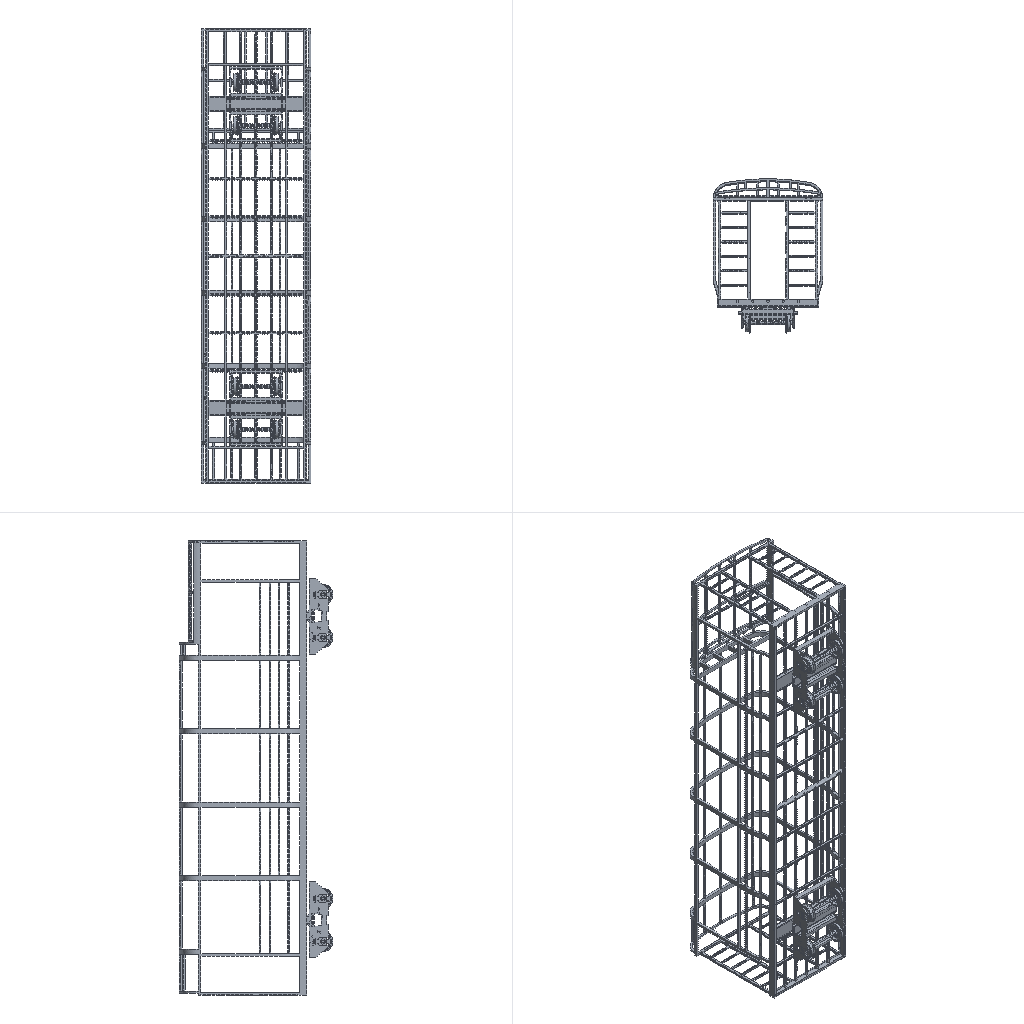Simulation study | ansys workbench
Set-up summary:
category,name,step,type,value,unit,region
solver,ansys_workbench
units,mm-N-s-tonne (MPa),,stated,"/units,MPA"
analysis,LS1,,static
load_step,LS1,LS1,static,nsubst=1; time=1
mesh,nodes,,,844923
mesh,elements,,,483421
element_type,SOLID187,,,440747
element_type,CONTA174,,,27682
element_type,TARGE170,,,10972
element_type,SOLID186,,,4020
material,Structural Steel,,E,200000,tonne s^-2 mm^-1
material,Structural Steel,,nu,0.3
material,Structural Steel,,density,7.85e-09,tonne mm^-3
material,Structural Steel,,conductivity,60.5,tonne mm s^-3 C^-1
material,Structural Steel,,specific_heat,4.34e+08,mm^2 s^-2 C^-1
material,Structural Steel,,cte,1.2e-05,C^-1
material,Structural Steel,,permeability,10000
material,Structural Steel,,resistivity,0.00017,ohm mm
load,,LS1,force,"13770 [dir=(-1, 0, 0) n=3]",,all
load,ACEL,LS1,gravity (ACEL; gravity acts opposite),"9806.65 [dir=(0, -1, 0)]",,all
bc,Constant Zero Displacement X,model,fixed,[dofs=UX],,_DISPZEROUX
bc,Constant Zero Displacement Y,model,fixed,[dofs=UY],,_DISPZEROUY
bc,Constant Zero Displacement Z,model,fixed,[dofs=UZ],,_DISPZEROUZ
contact,Contact Region 10,,bonded (always),element=CONTA174
contact,Contact Region 11,,bonded (always),element=CONTA174
contact,Contact Region 12,,bonded (always),element=CONTA174
contact,Contact Region 13,,bonded (always),element=CONTA174
contact,Contact Region 14,,bonded (always),element=CONTA174
contact,Contact Region 15,,bonded (always),element=CONTA174
contact,Contact Region 16,,bonded (always),element=CONTA174
contact,Contact Region 17,,bonded (always),element=CONTA174
contact,Contact Region 18,,bonded (always),element=CONTA174
contact,Contact Region 19,,bonded (always),element=CONTA174
contact,Contact Region 20,,bonded (always),element=CONTA174
contact,Contact Region 21,,bonded (always),element=CONTA174
contact,Contact Region 22,,bonded (always),element=CONTA174
contact,Contact Region 23,,bonded (always),element=CONTA174
contact,Contact Region 24,,bonded (always),element=CONTA174
contact,Contact Region 25,,bonded (always),element=CONTA174
contact,Contact Region 26,,bonded (always),element=CONTA174
contact,Contact Region 27,,bonded (always),element=CONTA174
contact,Contact Region 28,,bonded (always),element=CONTA174
contact,Contact Region 29,,bonded (always),element=CONTA174
contact,Contact Region 30,,bonded (always),element=CONTA174
contact,Contact Region 31,,bonded (always),element=CONTA174
contact,Contact Region 32,,bonded (always),element=CONTA174
contact,Contact Region 33,,bonded (always),element=CONTA174
contact,Contact Region 34,,bonded (always),element=CONTA174
contact,Contact Region 35,,bonded (always),element=CONTA174
contact,Contact Region 36,,bonded (always),element=CONTA174
contact,Contact Region 37,,bonded (always),element=CONTA174
contact,Contact Region 38,,bonded (always),element=CONTA174
contact,Contact Region 39,,bonded (always),element=CONTA174
contact,Contact Region 40,,bonded (always),element=CONTA174
contact,Contact Region 41,,bonded (always),element=CONTA174
contact,Contact Region 42,,bonded (always),element=CONTA174
contact,Contact Region 43,,bonded (always),element=CONTA174
contact,Contact Region 44,,bonded (always),element=CONTA174
contact,Contact Region 45,,bonded (always),element=CONTA174
contact,Contact Region 46,,bonded (always),element=CONTA174
contact,Contact Region 47,,bonded (always),element=CONTA174
contact,Contact Region 48,,bonded (always),element=CONTA174
contact,Contact Region 49,,bonded (always),element=CONTA174
contact,Contact Region 50,,bonded (always),element=CONTA174
contact,Contact Region 51,,bonded (always),element=CONTA174
contact,Contact Region 52,,bonded (always),element=CONTA174
contact,Contact Region 53,,bonded (always),element=CONTA174
contact,Contact Region 54,,bonded (always),element=CONTA174
contact,Contact Region 55,,bonded (always),element=CONTA174
contact,Contact Region 56,,bonded (always),element=CONTA174
contact,Contact Region 57,,bonded (always),element=CONTA174
contact,Contact Region 58,,bonded (always),element=CONTA174
contact,Contact Region 59,,bonded (always),element=CONTA174
contact,Contact Region 60,,bonded (always),element=CONTA174
contact,Contact Region 61,,bonded (always),element=CONTA174
contact,Contact Region 62,,bonded (always),element=CONTA174
contact,Contact Region 63,,bonded (always),element=CONTA174
contact,Contact Region 64,,bonded (always),element=CONTA174
contact,Contact Region 65,,bonded (always),element=CONTA174
contact,Contact Region 66,,bonded (always),element=CONTA174
contact,Contact Region 67,,bonded (always),element=CONTA174
contact,Contact Region 68,,bonded (always),element=CONTA174
contact,Contact Region 69,,bonded (always),element=CONTA174
contact,Contact Region 70,,bonded (always),element=CONTA174
contact,Contact Region 71,,bonded (always),element=CONTA174
contact,Contact Region 72,,bonded (always),element=CONTA174
contact,Contact Region 73,,bonded (always),element=CONTA174
contact,Contact Region 74,,bonded (always),element=CONTA174
contact,Contact Region 75,,bonded (always),element=CONTA174
contact,Contact Region 76,,bonded (always),element=CONTA174
contact,Contact Region 77,,bonded (always),element=CONTA174
contact,Contact Region 78,,bonded (always),element=CONTA174
contact,Contact Region 79,,bonded (always),element=CONTA174
contact,Contact Region 80,,bonded (always),element=CONTA174
contact,Contact Region 81,,bonded (always),element=CONTA174
contact,Contact Region 82,,bonded (always),element=CONTA174
contact,Contact Region 83,,bonded (always),element=CONTA174
contact,Contact Region 84,,bonded (always),element=CONTA174
contact,Contact Region 85,,bonded (always),element=CONTA174
contact,Contact Region 86,,bonded (always),element=CONTA174
contact,Contact Region 87,,bonded (always),element=CONTA174
contact,Contact Region 88,,bonded (always),element=CONTA174
contact,Contact Region 89,,bonded (always),element=CONTA174
contact,Contact Region 90,,bonded (always),element=CONTA174
contact,Contact Region 91,,bonded (always),element=CONTA174
contact,Contact Region 92,,bonded (always),element=CONTA174
contact,Contact Region 93,,bonded (always),element=CONTA174
contact,Contact Region 94,,bonded (always),element=CONTA174
contact,Contact Region 95,,bonded (always),element=CONTA174
contact,Contact Region 96,,bonded (always),element=CONTA174
contact,Contact Region 97,,bonded (always),element=CONTA174
contact,Contact Region 98,,bonded (always),element=CONTA174
contact,Contact Region 99,,bonded (always),element=CONTA174
contact,Contact Region 100,,bonded (always),element=CONTA174
contact,Contact Region 101,,bonded (always),element=CONTA174
contact,Contact Region 102,,bonded (always),element=CONTA174
contact,Contact Region 103,,bonded (always),element=CONTA174
contact,Contact Region 104,,bonded (always),element=CONTA174
contact,Contact Region 105,,bonded (always),element=CONTA174
contact,Contact Region 106,,bonded (always),element=CONTA174
contact,Contact Region 107,,bonded (always),element=CONTA174
contact,Contact Region 108,,bonded (always),element=CONTA174
contact,Contact Region 109,,bonded (always),element=CONTA174
contact,Contact Region 110,,bonded (always),element=CONTA174
contact,Contact Region 111,,bonded (always),element=CONTA174
contact,Contact Region 112,,bonded (always),element=CONTA174
contact,Contact Region 113,,bonded (always),element=CONTA174
contact,Contact Region 114,,bonded (always),element=CONTA174
contact,Contact Region 115,,bonded (always),element=CONTA174
contact,Contact Region 116,,bonded (always),element=CONTA174
contact,Contact Region 117,,bonded (always),element=CONTA174
contact,Contact Region 118,,bonded (always),element=CONTA174
contact,Contact Region 119,,bonded (always),element=CONTA174
contact,Contact Region 120,,bonded (always),element=CONTA174
contact,contact 112,,bonded (always),element=CONTA174
contact,contact 113,,bonded (always),element=CONTA174
contact,contact 114,,bonded (always),element=CONTA174
named_set,_DISPZEROUX,,node,2976
named_set,_DISPZEROUY,,node,2976
named_set,_DISPZEROUZ,,node,1488
Ansys APDL input file, long lists of numbers shortened:
/batch
/config,noeldb,1     ! force off writing results to database
*get,_wallstrt,active,,time,wall
! ANSYS input file written by Workbench version 2021 R1
! File used for geometry attach:
/title,_______--____ 5 (F5)
! ****** Begin Custom Load Command Snippet ******
/COM, ACT Extensions:
/COM,     LSDYNA, 2021.1
/COM,
! ****** End   Custom Load Command Snippet ******
*DIM,_wb_ProjectScratch_dir,string,248
_wb_ProjectScratch_dir(1) = ''
*DIM,_wb_SolverFiles_dir,string,248
_wb_SolverFiles_dir(1) = ''
*DIM,_wb_userfiles_dir,string,248
_wb_userfiles_dir(1) = ''
/com,--- Data in consistent NMM units. See Solving Units in the help system for more information.
/units,MPA
/nopr
/wb,file,start              !  signify a WB generated input file
/prep7
! Turn off shape checking because checks already performed inside WB mesher.
! See help system for more information.
SHPP,OFF,,NOWARN
/nolist
etcon,set             ! allow ANSYS to choose best KEYOP's for 180x elements, resets any applicable keyopt to MAPDL defaults
/com,*********** Nodes for the whole assembly ***********
nblock,3,,929390
(1i9,3e20.9e3)
        1     5.000000000E+02    -2.700000000E+02     8.500000000E+01
! (844899 more lines like these left out)
-1
/com,*********** Nodes for all Remote Points ***********
nblock,3
(1i9,3e20.9e3)
   844901     0.000000000E+00    -4.570000000E+02     1.250000000E+03
! (22 more lines like these left out)
-1
/wb,elem,start            !  set before creation of elements
/com,*********** Elements for Body 1 "____-0|NONE" ***********
et,1,187
eblock,19,solid,,219008
(19i9)
        1        1        1        1        0        0        0        0       10        0   225760   496373   499028   502293   501893   835194   841376   835201   835199
! (438015 more lines like these left out)
-1
/com,*********** Elements for Body 2 "______|NONE" ***********
et,2,186
keyo,2,2,1          ! set full integration on SOLID186
eblock,19,solid,,316
(19i9)
        2        2        2        2        0        0        0        0       20        0      914     6556     6586     6589     6565     6931     6901     6898     6922
! (631 more lines like these left out)
-1
/com,*********** Elements for Body 3 "______|NONE[2]" ***********
et,3,186
keyo,3,2,1          ! set full integration on SOLID186
eblock,19,solid,,316
(19i9)
        3        3        3        3        0        0        0        0       20        0     1663    12147    12177    12180    12156    12522    12492    12489    12513
! (631 more lines like these left out)
-1
/com,*********** Elements for Body 4 "______|NONE[3]" ***********
et,4,186
keyo,4,2,1          ! set full integration on SOLID186
eblock,19,solid,,420
(19i9)
        4        4        4        4        0        0        0        0       20        0     1243     9304     9447     9466     9364     9345     9446     9485     9365
! (839 more lines like these left out)
-1
/com,*********** Elements for Body 5 "______|NONE[4]" ***********
et,5,186
keyo,5,2,1          ! set full integration on SOLID186
eblock,19,solid,,420
(19i9)
        5        5        5        5        0        0        0        0       20        0      481     3579     3722     3741     3639     3620     3721     3760     3640
! (839 more lines like these left out)
-1
! (55 more sections like these left out)
/wb,elem,end               !  done creating elements
/com,*********** Send User Defined Coordinate System(s) ***********
csys,0
toffst,273.15,  ! Temperature offset from absolute zero
/com,*********** Set Reference Temperature ***********
tref,22.
/wb,mat,start              !  starting to send materials
/com,*********** Send Materials ***********
Temperature = 'TEMP' ! Temperature
MP,DENS,1,7.85e-09,	! tonne mm^-3
MP,ALPX,1,1.2e-05,	! C^-1
MP,C,1,434000000,	! mm^2 s^-2 C^-1
MP,KXX,1,60.5,	! tonne mm s^-3 C^-1
MP,RSVX,1,0.00017,	! ohm mm
MP,EX,1,200000,	! tonne s^-2 mm^-1
MP,NUXY,1,0.3,
MP,MURX,1,10000,
Temperature = 'TEMP' ! Temperature
MP,DENS,2,7.85e-09,	! tonne mm^-3
MP,ALPX,2,1.2e-05,	! C^-1
MP,C,2,434000000,	! mm^2 s^-2 C^-1
MP,KXX,2,60.5,	! tonne mm s^-3 C^-1
MP,RSVX,2,0.00017,	! ohm mm
MP,EX,2,200000,	! tonne s^-2 mm^-1
MP,NUXY,2,0.3,
MP,MURX,2,10000,
Temperature = 'TEMP' ! Temperature
MP,DENS,3,7.85e-09,	! tonne mm^-3
MP,ALPX,3,1.2e-05,	! C^-1
MP,C,3,434000000,	! mm^2 s^-2 C^-1
MP,KXX,3,60.5,	! tonne mm s^-3 C^-1
MP,RSVX,3,0.00017,	! ohm mm
MP,EX,3,200000,	! tonne s^-2 mm^-1
MP,NUXY,3,0.3,
MP,MURX,3,10000,
Temperature = 'TEMP' ! Temperature
MP,DENS,4,7.85e-09,	! tonne mm^-3
MP,ALPX,4,1.2e-05,	! C^-1
MP,C,4,434000000,	! mm^2 s^-2 C^-1
MP,KXX,4,60.5,	! tonne mm s^-3 C^-1
MP,RSVX,4,0.00017,	! ohm mm
MP,EX,4,200000,	! tonne s^-2 mm^-1
MP,NUXY,4,0.3,
MP,MURX,4,10000,
Temperature = 'TEMP' ! Temperature
MP,DENS,5,7.85e-09,	! tonne mm^-3
MP,ALPX,5,1.2e-05,	! C^-1
MP,C,5,434000000,	! mm^2 s^-2 C^-1
MP,KXX,5,60.5,	! tonne mm s^-3 C^-1
MP,RSVX,5,0.00017,	! ohm mm
MP,EX,5,200000,	! tonne s^-2 mm^-1
MP,NUXY,5,0.3,
MP,MURX,5,10000,
Temperature = 'TEMP' ! Temperature
MP,DENS,6,7.85e-09,	! tonne mm^-3
MP,ALPX,6,1.2e-05,	! C^-1
MP,C,6,434000000,	! mm^2 s^-2 C^-1
MP,KXX,6,60.5,	! tonne mm s^-3 C^-1
MP,RSVX,6,0.00017,	! ohm mm
MP,EX,6,200000,	! tonne s^-2 mm^-1
MP,NUXY,6,0.3,
MP,MURX,6,10000,
Temperature = 'TEMP' ! Temperature
MP,DENS,7,7.85e-09,	! tonne mm^-3
MP,ALPX,7,1.2e-05,	! C^-1
MP,C,7,434000000,	! mm^2 s^-2 C^-1
MP,KXX,7,60.5,	! tonne mm s^-3 C^-1
MP,RSVX,7,0.00017,	! ohm mm
MP,EX,7,200000,	! tonne s^-2 mm^-1
MP,NUXY,7,0.3,
MP,MURX,7,10000,
Temperature = 'TEMP' ! Temperature
MP,DENS,8,7.85e-09,	! tonne mm^-3
MP,ALPX,8,1.2e-05,	! C^-1
MP,C,8,434000000,	! mm^2 s^-2 C^-1
MP,KXX,8,60.5,	! tonne mm s^-3 C^-1
MP,RSVX,8,0.00017,	! ohm mm
MP,EX,8,200000,	! tonne s^-2 mm^-1
MP,NUXY,8,0.3,
MP,MURX,8,10000,
Temperature = 'TEMP' ! Temperature
MP,DENS,9,7.85e-09,	! tonne mm^-3
MP,ALPX,9,1.2e-05,	! C^-1
MP,C,9,434000000,	! mm^2 s^-2 C^-1
MP,KXX,9,60.5,	! tonne mm s^-3 C^-1
MP,RSVX,9,0.00017,	! ohm mm
MP,EX,9,200000,	! tonne s^-2 mm^-1
! (461 more lines like these left out)
/wb,mat,end                !  done sending materials
!************************* Model Summary ********************
!____-0|NONE,	结构钢,	matid,	1
!______|NONE,	结构钢,	matid,	2
!______|NONE[2],	结构钢,	matid,	3
! (59 more lines like these left out)
*get,_xmin,node,,mnloc,x
*get,_ymin,node,,mnloc,y
*get,_zmin,node,,mnloc,z
*get,_xmax,node,,mxloc,x
*get,_ymax,node,,mxloc,y
*get,_zmax,node,,mxloc,z
_ASMDIAG=(_xmax-_xmin)*(_xmax-_xmin)+(_ymax-_ymin)*(_ymax-_ymin)+(_zmax-_zmin)*(_zmax-_zmin)
_ASMDIAG=SQRT(_ASMDIAG)
/wb,contact,start          !  starting to send contact
/com,*********** Create Contact "接触区域 10" ***********
/com,            Real Constant Set For Above Contact Is 62 & 61
*set,tid,62
*set,cid,61
r,tid
r,cid
et,tid,170
et,cid,174
eblock,10,,,42
(15i9)
   662855       62       62       62        0     6714     6723     6734     6734     7990     8015     6734     7992
! (41 more lines like these left out)
-1
eblock,10,,,42
(15i9)
   662897       61       61       61        0     6714     6723     6734     6734     7990     8015     6734     7992
! (41 more lines like these left out)
-1
eblock,10,,,21
(15i9)
   662939       61       62       61        0     9885    10045     9244     9244    11813    10203     9244    10202
! (20 more lines like these left out)
-1
eblock,10,,,21
(15i9)
   662960       62       61       62        0     9885    10045     9244     9244    11813    10203     9244    10202
! (20 more lines like these left out)
-1
keyo,cid,8,2               ! auto create asymmetric contact (from Program Controlled setting)
keyo,cid,10,0              ! adjust contact stiffness each NR iteration (from Program Controlled setting)
keyo,cid,12,5              ! bonded always
keyo,cid,18,1              ! small sliding turned on by application
keyo,cid,2,0               ! augmented Lagrange (from Program Controlled setting)
keyo,cid,4,0               ! on Gauss point (from Program Controlled setting)
keyo,cid,9,1               ! ignore initial gaps/penetration
keyo,cid,7,0               ! No Prediction
rmod,tid,3,10.      ! FKN
rmod,tid,5,0.       ! ICONT
rmod,tid,6,0.       ! PINB
rmod,tid,10,0.      ! CNOF
rmod,tid,12,0.      ! FKT
rmod,tid,36,14962   ! WB DSID
rmod,cid,3,10.      ! FKN
rmod,cid,5,0.       ! ICONT
rmod,cid,6,0.       ! PINB
rmod,cid,10,0.      ! CNOF
rmod,cid,12,0.      ! FKT
rmod,cid,36,14962   ! WB DSID
/com,*********** Create Contact "接触区域 11" ***********
/com,            Real Constant Set For Above Contact Is 64 & 63
*set,tid,64
*set,cid,63
r,tid
r,cid
et,tid,170
et,cid,174
eblock,10,,,48
(15i9)
   662981       64       64       64        0     6688     6733     6595     6595     7938     7613     6595     7610
! (47 more lines like these left out)
-1
eblock,10,,,48
(15i9)
   663029       63       63       63        0     6688     6733     6595     6595     7938     7613     6595     7610
! (47 more lines like these left out)
-1
eblock,10,,,21
(15i9)
   663077       63       64       63        0     3534     3522     3523     3523     4485     4484     3523     4488
! (20 more lines like these left out)
-1
eblock,10,,,21
(15i9)
   663098       64       63       64        0     3534     3522     3523     3523     4485     4484     3523     4488
! (20 more lines like these left out)
-1
keyo,cid,8,2               ! auto create asymmetric contact (from Program Controlled setting)
keyo,cid,10,0              ! adjust contact stiffness each NR iteration (from Program Controlled setting)
keyo,cid,12,5              ! bonded always
keyo,cid,18,1              ! small sliding turned on by application
keyo,cid,2,0               ! augmented Lagrange (from Program Controlled setting)
keyo,cid,4,0               ! on Gauss point (from Program Controlled setting)
keyo,cid,9,1               ! ignore initial gaps/penetration
keyo,cid,7,0               ! No Prediction
rmod,tid,3,10.      ! FKN
rmod,tid,5,0.       ! ICONT
rmod,tid,6,0.       ! PINB
rmod,tid,10,0.      ! CNOF
rmod,tid,12,0.      ! FKT
rmod,tid,36,14965   ! WB DSID
rmod,cid,3,10.      ! FKN
rmod,cid,5,0.       ! ICONT
rmod,cid,6,0.       ! PINB
rmod,cid,10,0.      ! CNOF
rmod,cid,12,0.      ! FKT
rmod,cid,36,14965   ! WB DSID
/com,*********** Create Contact "接触区域 12" ***********
/com,            Real Constant Set For Above Contact Is 66 & 65
*set,tid,66
*set,cid,65
r,tid
r,cid
et,tid,170
et,cid,174
eblock,10,,,16
(15i9)
   663119       66       66       66        0     6741     6708     6696     6709     7977     7955     7956     7980
! (15 more lines like these left out)
-1
eblock,10,,,16
(15i9)
   663135       65       65       65        0     6741     6708     6696     6709     7977     7955     7956     7980
! (15 more lines like these left out)
-1
eblock,10,,,12
(15i9)
   663151       65       66       65        0     1744     1745     1761     1756     2255     2259     2289     2257
! (11 more lines like these left out)
-1
eblock,10,,,12
(15i9)
   663163       66       65       66        0     1744     1745     1761     1756     2255     2259     2289     2257
! (11 more lines like these left out)
-1
keyo,cid,8,2               ! auto create asymmetric contact (from Program Controlled setting)
keyo,cid,10,0              ! adjust contact stiffness each NR iteration (from Program Controlled setting)
keyo,cid,12,5              ! bonded always
keyo,cid,18,1              ! small sliding turned on by application
keyo,cid,2,0               ! augmented Lagrange (from Program Controlled setting)
keyo,cid,4,0               ! on Gauss point (from Program Controlled setting)
keyo,cid,9,1               ! ignore initial gaps/penetration
keyo,cid,7,0               ! No Prediction
rmod,tid,3,10.      ! FKN
rmod,tid,5,0.       ! ICONT
rmod,tid,6,0.       ! PINB
rmod,tid,10,0.      ! CNOF
rmod,tid,12,0.      ! FKT
rmod,tid,36,14968   ! WB DSID
rmod,cid,3,10.      ! FKN
rmod,cid,5,0.       ! ICONT
rmod,cid,6,0.       ! PINB
rmod,cid,10,0.      ! CNOF
rmod,cid,12,0.      ! FKT
rmod,cid,36,14968   ! WB DSID
/com,*********** Create Contact "接触区域 13" ***********
/com,            Real Constant Set For Above Contact Is 68 & 67
*set,tid,68
*set,cid,67
r,tid
r,cid
et,tid,170
et,cid,174
eblock,10,,,15
(15i9)
   663175       68       68       68        0     6738     6691     6692     6739     7945     7944     7948     8042
! (14 more lines like these left out)
-1
eblock,10,,,15
(15i9)
   663190       67       67       67        0     6738     6691     6692     6739     7945     7944     7948     8042
! (14 more lines like these left out)
-1
eblock,10,,,12
(15i9)
   663205       67       68       67        0       21       16        4        5      549      517      515      519
! (11 more lines like these left out)
-1
eblock,10,,,12
(15i9)
   663217       68       67       68        0       21       16        4        5      549      517      515      519
! (11 more lines like these left out)
-1
keyo,cid,8,2               ! auto create asymmetric contact (from Program Controlled setting)
keyo,cid,10,0              ! adjust contact stiffness each NR iteration (from Program Controlled setting)
keyo,cid,12,5              ! bonded always
keyo,cid,18,1              ! small sliding turned on by application
keyo,cid,2,0               ! augmented Lagrange (from Program Controlled setting)
keyo,cid,4,0               ! on Gauss point (from Program Controlled setting)
keyo,cid,9,1               ! ignore initial gaps/penetration
keyo,cid,7,0               ! No Prediction
rmod,tid,3,10.      ! FKN
rmod,tid,5,0.       ! ICONT
rmod,tid,6,0.       ! PINB
rmod,tid,10,0.      ! CNOF
rmod,tid,12,0.      ! FKT
rmod,tid,36,14971   ! WB DSID
rmod,cid,3,10.      ! FKN
rmod,cid,5,0.       ! ICONT
rmod,cid,6,0.       ! PINB
rmod,cid,10,0.      ! CNOF
rmod,cid,12,0.      ! FKT
rmod,cid,36,14971   ! WB DSID
/com,*********** Create Contact "接触区域 14" ***********
/com,            Real Constant Set For Above Contact Is 70 & 69
*set,tid,70
*set,cid,69
r,tid
r,cid
et,tid,170
et,cid,174
eblock,10,,,33
(15i9)
   663229       70       70       70        0     7129     7127     7128     7133     8908     8907     8909     8911
! (32 more lines like these left out)
-1
eblock,10,,,33
(15i9)
   663262       69       69       69        0     7129     7127     7128     7133     8908     8907     8909     8911
! (32 more lines like these left out)
-1
eblock,10,,,170
(15i9)
   663295       69       70       69        0    17468    17488    17473    17473    26290    26306    17473    26287
! (169 more lines like these left out)
-1
eblock,10,,,170
(15i9)
   663465       70       69       70        0    17468    17488    17473    17473    26290    26306    17473    26287
! (169 more lines like these left out)
-1
keyo,cid,8,2               ! auto create asymmetric contact (from Program Controlled setting)
keyo,cid,10,0              ! adjust contact stiffness each NR iteration (from Program Controlled setting)
keyo,cid,12,5              ! bonded always
keyo,cid,18,1              ! small sliding turned on by application
keyo,cid,2,0               ! augmented Lagrange (from Program Controlled setting)
keyo,cid,4,0               ! on Gauss point (from Program Controlled setting)
keyo,cid,9,1               ! ignore initial gaps/penetration
keyo,cid,7,0               ! No Prediction
rmod,tid,3,10.      ! FKN
rmod,tid,5,0.       ! ICONT
rmod,tid,6,0.       ! PINB
rmod,tid,10,0.      ! CNOF
rmod,tid,12,0.      ! FKT
rmod,tid,36,14974   ! WB DSID
rmod,cid,3,10.      ! FKN
rmod,cid,5,0.       ! ICONT
rmod,cid,6,0.       ! PINB
rmod,cid,10,0.      ! CNOF
rmod,cid,12,0.      ! FKT
rmod,cid,36,14974   ! WB DSID
! (106 more sections like these left out)
/wb,contact,end            !  done creating contacts
/golist
/wb,load,start             !  starting to send loads
/com,******* Constant Zero Displacement X *******
CMBLOCK,_DISPZEROUX,NODE,     2976
(8i10)
     33525     33526     33527     33528     33529     33530     33531     33532
! (371 more lines like these left out)
cmsel,s,_DISPZEROUX
d,all,ux,0
nsel,all
/com,******* Constant Zero Displacement Y *******
CMBLOCK,_DISPZEROUY,NODE,     2976
(8i10)
     33525     33526     33527     33528     33529     33530     33531     33532
! (371 more lines like these left out)
cmsel,s,_DISPZEROUY
d,all,uy,0
nsel,all
/com,******* Constant Zero Displacement Z *******
CMBLOCK,_DISPZEROUZ,NODE,     1488
(8i10)
     33525     33526     33527     33528     33529     33530     33531     33532
! (185 more lines like these left out)
cmsel,s,_DISPZEROUZ
d,all,uz,0
nsel,all
/com,*********** Create Remote Point "内部远程点 17" ***********
! -------- Remote Point Used by "乘客重量" --------
*set,tid,284
*set,cid,283
et,cid,174
et,tid,170
keyo,tid,2,1               ! Don't fix the pilot node
keyo,tid,4,0               ! Activate all DOF's due to large deformation
keyo,cid,12,5              ! Bonded Contact
keyo,cid,4,1               ! Deformable RBE3 style load
keyo,cid,2,2               ! MPC style contact
eblock,10,,,6072
(15i9)
   684799      283      283      283        0   148608   149004   149355   149355   346755   349666   149355   346758
! (6071 more lines like these left out)
-1
*set,_npilot,844917
_npilot15533=_npilot
type,tid
mat ,cid
real,cid
tshape,pilo
en,690871,_npilot
tshape
/com,*********** Create Remote Point "内部远程点 18" ***********
! -------- Remote Point Used by "点质量 " --------
*set,tid,286
*set,cid,285
et,cid,174
et,tid,170
keyo,tid,2,1               ! Don't fix the pilot node
keyo,tid,4,0               ! Activate all DOF's due to large deformation
keyo,cid,12,5              ! Bonded Contact
keyo,cid,4,1               ! Deformable RBE3 style load
keyo,cid,2,2               ! MPC style contact
eblock,10,,,6072
(15i9)
   690872      285      285      285        0   148608   149004   149355   149355   346755   349666   149355   346758
! (6071 more lines like these left out)
-1
*set,_npilot,844918
_npilot15580=_npilot
type,tid
mat ,cid
real,cid
tshape,pilo
en,696944,_npilot
tshape
/com,*********** Create Remote Point "内部远程点 22" ***********
! -------- Remote Point Used by "侧向风力" --------
*set,tid,288
*set,cid,287
et,cid,174
et,tid,170
keyo,tid,2,1               ! Don't fix the pilot node
keyo,tid,4,0               ! Activate all DOF's due to large deformation
keyo,cid,12,5              ! Bonded Contact
keyo,cid,4,1               ! Deformable RBE3 style load
keyo,cid,2,2               ! MPC style contact
eblock,10,,,4566
(15i9)
   696945      287      287      287        0   463974   464095   441846   441846   702069   546199   441846   546197
! (4565 more lines like these left out)
-1
*set,_npilot,844927
_npilot15664=_npilot
type,tid
mat ,cid
real,cid
tshape,pilo
en,701511,_npilot
tshape
/com,*********** Construct Remote Force ***********
*DIM,_loadvari15663x,TABLE,2,1,1,TIME,
! Time values
_loadvari15663x(1,0,1) = 0.
_loadvari15663x(2,0,1) = 1.
! Load values
_loadvari15663x(1,1,1) = 0.
_loadvari15663x(2,1,1) = -13770.
*DIM,_loadvari15663y,TABLE,2,1,1,TIME,
! Time values
_loadvari15663y(1,0,1) = 0.
_loadvari15663y(2,0,1) = 1.
! Load values
_loadvari15663y(1,1,1) = 0.
_loadvari15663y(2,1,1) = 0.
*DIM,_loadvari15663z,TABLE,2,1,1,TIME,
! Time values
_loadvari15663z(1,0,1) = 0.
_loadvari15663z(2,0,1) = 1.
! Load values
_loadvari15663z(1,1,1) = 0.
_loadvari15663z(2,1,1) = 0.
/com,*********** Construct Remote Mass Using Remote Attachment ***********
*set,_tid,289
et,_tid,21           ! MASS21 element
type,_tid
mat ,_tid
real,_tid
keyo,_tid,3,2        ! 3d mass without rotary inertia
r,_tid,2.8
en,701512,844917
/com,*********** Construct Remote Mass Using Remote Attachment ***********
*set,_tid,290
et,_tid,21           ! MASS21 element
type,_tid
mat ,_tid
real,_tid
keyo,_tid,3,2        ! 3d mass without rotary inertia
r,_tid,0.45
en,701513,844918
/gst,on,on
fini
*get,_numnode,node,0,count
*get,_numelem,elem,0,count
*get, _MAXELEMNUM, elem, 0, NUM, MAX
*get, _MAXNODENUM, node, 0, NUM, MAX
*get, _MAXELEMTYPE, etyp, 0, NUM, MAX
*get, _MAXREALCONST, real, 0, NUM, MAX
/go
/wb,load,end               !  done creating loads
/com,--- Number of total nodes = %_numnode%
/com,--- Number of contact elements = 38654
/com,--- Number of spring elements = 0
/com,--- Number of bearing elements = 0
/com,--- Number of solid elements = 444767
/com,--- Number of condensed parts = 0
/com,--- Number of total elements = %_numelem%
*get,_wallbsol,active,,time,wall
/com,****************************************************************************
/com,*************************    SOLUTION       ********************************
/com,****************************************************************************
/solu
antype,0                   ! static analysis
nlgeom,on                  ! Turn on Large Deformation Effects
_thickRatio=0.1     ! Ratio of thick parts in the model
eqsl,sparse,,,,,1
cntr,print,1               ! print out contact info and also make no initial contact an error
cntr,out,yes               ! write contact output to file.cmn due to many contact pairs present
dmpoption,emat,no             ! Don't combine emat file for DANSYS
dmpoption,esav,no             ! Don't combine esav file for DANSYS
nldiag,cont,iter           ! print out contact info each equilibrium iteration
rescontrol,define,last,last,,dele	   ! Program Controlled
/com,****************************************************
/com,******************* SOLVE FOR LS 1 OF 1 ****************
nsel,s,node,,844927
f,all,fx,%_loadvari15663x%
f,all,fy,%_loadvari15663y%
f,all,fz,%_loadvari15663z%
nsel,all
acel,0.,9806.65,0.
/nopr
/gopr
/nolist
autots,on                  ! Workbench Program Controlled automatic time stepping
nsub,1,10,1                ! due to presence of general nonlinear
time,1.
outres,erase
outres,all,none
outres,nsol,all,
outres,rsol,all
outres,eangl,all
outres,etmp,all
outres,veng,all
outres,strs,all,
outres,epel,all,
outres,eppl,all,
outres,cont,all,
! *********** WB SOLVE COMMAND ***********
! check interactive state
*get,ANSINTER_,active,,int
*if,ANSINTER_,ne,0,then
/eof
*endif
solve
/com *************** Write FE CONNECTORS *********
CEWRITE,file,ce,,INTE
/com,****************************************************
/com,*************** FINISHED SOLVE FOR LS 1 *************
*get,_wallasol,active,,time,wall
/nopr
*get,_numnode,node,0,count
*get,_numelem,elem,0,count
*get, _MAXELEMNUM, elem, 0, NUM, MAX
*get, _MAXNODENUM, node, 0, NUM, MAX,,,INTERNAL
*get, _MAXELEMTYPE, etyp, 0, NUM, MAX
*get, _MAXREALCONST, real, 0, NUM, MAX
/gopr
/post1
xmlo,ENCODING,ISO-8859-1
xmlo,parm
/xml,parm,xml
fini
/gopr
*get,_walldone,active,,time,wall
_preptime=(_wallbsol-_wallstrt)*3600
_solvtime=(_wallasol-_wallbsol)*3600
_posttime=(_walldone-_wallasol)*3600
_totaltim=(_walldone-_wallstrt)*3600
*get,_dlbratio,active,0,solu,dlbr
*get,_combtime,active,0,solu,comb
/com,--- Total number of nodes = %_numnode%
/com,--- Total number of elements = %_numelem%
/com,--- Element load balance ratio = %_dlbratio%
/com,--- Time to combine distributed files = %_combtime%
/wb,file,end               ! done with WB generated input
Results summary:
result,analyses[0].index,,,1
result,analyses[0].system,,,SYS-5
result,analyses[0].deck,,,deck.dat
result,analyses[0].solve_status,,,completed
result,analyses[0].analysis_type,,,static
result,analyses[0].physics,,,mechanical
result,analyses[0].unit_system,,,"NMM: mm, ton, N, s, mV, mA, degC"
result,analyses[0].n_sets,,,1
result,analyses[0].load_steps[0].set,set=1,,1
result,analyses[0].load_steps[0].time_or_freq,set=1,,1
result,analyses[0].load_steps[0].max_displacement_magnitude,set=1,,6.883
result,analyses[0].load_steps[0].max_von_mises_nodal,set=1,,161.293
result,analyses[0].load_steps[0].reaction_force_sum_xyz[1],set=1,,13770
result,analyses[0].load_steps[0].reaction_force_sum_xyz[2],set=1,,96375.6
result,analyses[0].load_steps[0].reaction_force_sum_xyz[3],set=1,,-0.01967
result,geometry_export[0][0],,,.step
result,geometry_export[0][1],,,ok
result,geometry_export[0][2],,,329